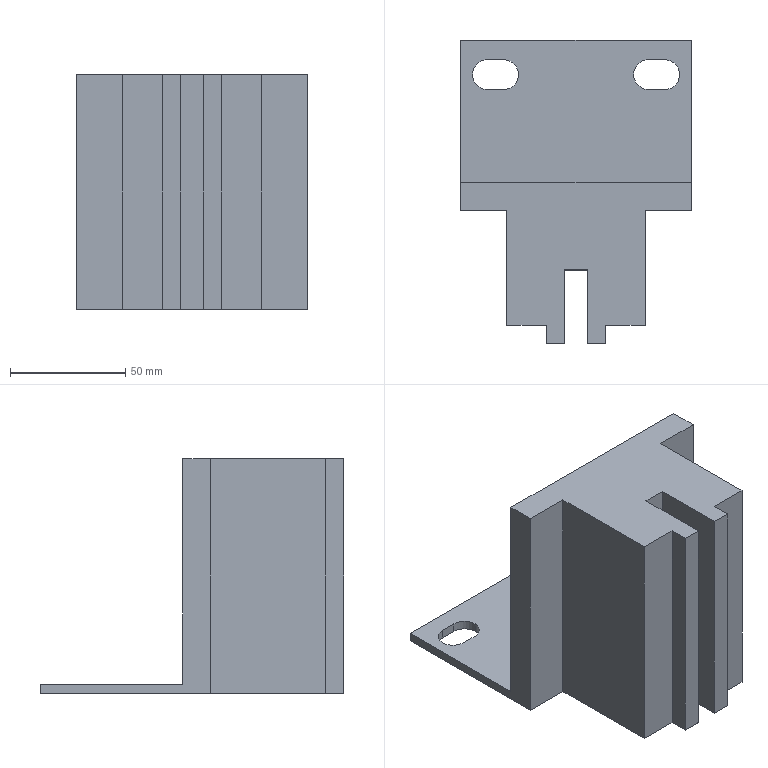Part | 1 solid | 30 faces | box 100 x 132 x 102 mm | volume 439986 mm3 | plane 24 | cylinder 6 | commonest cylinder face diameters 13 x6
STEP:
#1=CARTESIAN_POINT('',(45.,51.,0.));
#2=VERTEX_POINT('',#1);
#3=CARTESIAN_POINT('',(38.5,57.5,0.));
#4=VERTEX_POINT('',#3);
#5=CARTESIAN_POINT('',(38.5,51.,0.));
#6=DIRECTION('',(0.,0.,1.));
#7=DIRECTION('',(1.,0.,0.));
#8=AXIS2_PLACEMENT_3D('',#5,#6,#7);
#9=CIRCLE('',#8,6.5);
#10=EDGE_CURVE('',#2,#4,#9,.T.);
#11=ORIENTED_EDGE('',*,*,#10,.F.);
#12=CARTESIAN_POINT('',(45.,51.,4.));
#13=VERTEX_POINT('',#12);
#14=CARTESIAN_POINT('',(45.,51.,0.));
#15=DIRECTION('',(0.,0.,1.));
#16=VECTOR('',#15,1000.);
#17=LINE('',#14,#16);
#18=EDGE_CURVE('',#2,#13,#17,.T.);
#19=ORIENTED_EDGE('',*,*,#18,.T.);
#20=CARTESIAN_POINT('',(38.5,57.5,4.));
#21=VERTEX_POINT('',#20);
#22=CARTESIAN_POINT('',(38.5,51.,4.));
#23=DIRECTION('',(0.,0.,1.));
#24=DIRECTION('',(0.,1.,0.));
#25=AXIS2_PLACEMENT_3D('',#22,#23,#24);
#26=CIRCLE('',#25,6.5);
#27=EDGE_CURVE('',#13,#21,#26,.T.);
#28=ORIENTED_EDGE('',*,*,#27,.T.);
#29=CARTESIAN_POINT('',(38.5,57.5,0.));
#30=DIRECTION('',(0.,0.,1.));
#31=VECTOR('',#30,1000.);
#32=LINE('',#29,#31);
#33=EDGE_CURVE('',#4,#21,#32,.T.);
#34=ORIENTED_EDGE('',*,*,#33,.F.);
#35=EDGE_LOOP('',(#11,#19,#28,#34));
#36=FACE_OUTER_BOUND('',#35,.T.);
#37=CARTESIAN_POINT('',(38.5,51.,0.));
#38=DIRECTION('',(0.,0.,1.));
#39=DIRECTION('',(1.,0.,0.));
#40=AXIS2_PLACEMENT_3D('',#37,#38,#39);
#41=CYLINDRICAL_SURFACE('',#40,6.5);
#42=ADVANCED_FACE('',(#36),#41,.F.);
#43=CARTESIAN_POINT('',(-25.,51.,0.));
#44=VERTEX_POINT('',#43);
#45=CARTESIAN_POINT('',(-31.5,57.5,0.));
#46=VERTEX_POINT('',#45);
#47=CARTESIAN_POINT('',(-31.5,51.,0.));
#48=DIRECTION('',(0.,0.,1.));
#49=DIRECTION('',(-1.,0.,0.));
#50=AXIS2_PLACEMENT_3D('',#47,#48,#49);
#51=CIRCLE('',#50,6.5);
#52=EDGE_CURVE('',#44,#46,#51,.T.);
#53=ORIENTED_EDGE('',*,*,#52,.F.);
#54=CARTESIAN_POINT('',(-25.,51.,4.));
#55=VERTEX_POINT('',#54);
#56=CARTESIAN_POINT('',(-25.,51.,0.));
#57=DIRECTION('',(0.,0.,1.));
#58=VECTOR('',#57,1000.);
#59=LINE('',#56,#58);
#60=EDGE_CURVE('',#44,#55,#59,.T.);
#61=ORIENTED_EDGE('',*,*,#60,.T.);
#62=CARTESIAN_POINT('',(-31.5,57.5,4.));
#63=VERTEX_POINT('',#62);
#64=CARTESIAN_POINT('',(-31.5,51.,4.));
#65=DIRECTION('',(0.,0.,1.));
#66=DIRECTION('',(0.,1.,0.));
#67=AXIS2_PLACEMENT_3D('',#64,#65,#66);
#68=CIRCLE('',#67,6.5);
#69=EDGE_CURVE('',#55,#63,#68,.T.);
#70=ORIENTED_EDGE('',*,*,#69,.T.);
#71=CARTESIAN_POINT('',(-31.5,57.5,0.));
#72=DIRECTION('',(0.,0.,1.));
#73=VECTOR('',#72,1000.);
#74=LINE('',#71,#73);
#75=EDGE_CURVE('',#46,#63,#74,.T.);
#76=ORIENTED_EDGE('',*,*,#75,.F.);
#77=EDGE_LOOP('',(#53,#61,#70,#76));
#78=FACE_OUTER_BOUND('',#77,.T.);
#79=CARTESIAN_POINT('',(-31.5,51.,0.));
#80=DIRECTION('',(0.,0.,1.));
#81=DIRECTION('',(1.,0.,0.));
#82=AXIS2_PLACEMENT_3D('',#79,#80,#81);
#83=CYLINDRICAL_SURFACE('',#82,6.5);
#84=ADVANCED_FACE('',(#78),#83,.F.);
#85=CARTESIAN_POINT('',(5.,-66.,0.));
#86=VERTEX_POINT('',#85);
#87=CARTESIAN_POINT('',(13.,-66.,0.));
#88=VERTEX_POINT('',#87);
#89=CARTESIAN_POINT('',(-50.,-66.,0.));
#90=DIRECTION('',(1.,0.,0.));
#91=VECTOR('',#90,1000.);
#92=LINE('',#89,#91);
#93=EDGE_CURVE('',#86,#88,#92,.T.);
#94=ORIENTED_EDGE('',*,*,#93,.T.);
#95=CARTESIAN_POINT('',(13.,-66.,102.));
#96=VERTEX_POINT('',#95);
#97=CARTESIAN_POINT('',(13.,-66.,0.));
#98=DIRECTION('',(0.,0.,1.));
#99=VECTOR('',#98,1000.);
#100=LINE('',#97,#99);
#101=EDGE_CURVE('',#88,#96,#100,.T.);
#102=ORIENTED_EDGE('',*,*,#101,.T.);
#103=CARTESIAN_POINT('',(5.,-66.,102.));
#104=VERTEX_POINT('',#103);
#105=CARTESIAN_POINT('',(-50.,-66.,102.));
#106=DIRECTION('',(1.,0.,0.));
#107=VECTOR('',#106,1000.);
#108=LINE('',#105,#107);
#109=EDGE_CURVE('',#104,#96,#108,.T.);
#110=ORIENTED_EDGE('',*,*,#109,.F.);
#111=CARTESIAN_POINT('',(5.,-66.,102.));
#112=DIRECTION('',(0.,0.,-1.));
#113=VECTOR('',#112,1000.);
#114=LINE('',#111,#113);
#115=EDGE_CURVE('',#104,#86,#114,.T.);
#116=ORIENTED_EDGE('',*,*,#115,.T.);
#117=EDGE_LOOP('',(#94,#102,#110,#116));
#118=FACE_OUTER_BOUND('',#117,.T.);
#119=CARTESIAN_POINT('',(-50.,-66.,102.));
#120=DIRECTION('',(0.,1.,0.));
#121=DIRECTION('',(0.,0.,1.));
#122=AXIS2_PLACEMENT_3D('',#119,#120,#121);
#123=PLANE('',#122);
#124=ADVANCED_FACE('',(#118),#123,.F.);
#125=CARTESIAN_POINT('',(50.,-8.,102.));
#126=VERTEX_POINT('',#125);
#127=CARTESIAN_POINT('',(50.,4.,102.));
#128=VERTEX_POINT('',#127);
#129=CARTESIAN_POINT('',(50.,66.,102.));
#130=DIRECTION('',(0.,1.,0.));
#131=VECTOR('',#130,1000.);
#132=LINE('',#129,#131);
#133=EDGE_CURVE('',#126,#128,#132,.T.);
#134=ORIENTED_EDGE('',*,*,#133,.F.);
#135=CARTESIAN_POINT('',(50.,-8.,0.));
#136=VERTEX_POINT('',#135);
#137=CARTESIAN_POINT('',(50.,-8.,0.));
#138=DIRECTION('',(0.,0.,1.));
#139=VECTOR('',#138,1000.);
#140=LINE('',#137,#139);
#141=EDGE_CURVE('',#136,#126,#140,.T.);
#142=ORIENTED_EDGE('',*,*,#141,.F.);
#143=CARTESIAN_POINT('',(50.,66.,0.));
#144=VERTEX_POINT('',#143);
#145=CARTESIAN_POINT('',(50.,66.,0.));
#146=DIRECTION('',(0.,1.,0.));
#147=VECTOR('',#146,1000.);
#148=LINE('',#145,#147);
#149=EDGE_CURVE('',#136,#144,#148,.T.);
#150=ORIENTED_EDGE('',*,*,#149,.T.);
#151=CARTESIAN_POINT('',(50.,66.,4.));
#152=VERTEX_POINT('',#151);
#153=CARTESIAN_POINT('',(50.,66.,102.));
#154=DIRECTION('',(0.,0.,-1.));
#155=VECTOR('',#154,1000.);
#156=LINE('',#153,#155);
#157=EDGE_CURVE('',#152,#144,#156,.T.);
#158=ORIENTED_EDGE('',*,*,#157,.F.);
#159=CARTESIAN_POINT('',(50.,4.,4.));
#160=VERTEX_POINT('',#159);
#161=CARTESIAN_POINT('',(50.,66.,4.));
#162=DIRECTION('',(0.,-1.,0.));
#163=VECTOR('',#162,1000.);
#164=LINE('',#161,#163);
#165=EDGE_CURVE('',#152,#160,#164,.T.);
#166=ORIENTED_EDGE('',*,*,#165,.T.);
#167=CARTESIAN_POINT('',(50.,4.,102.));
#168=DIRECTION('',(0.,0.,1.));
#169=VECTOR('',#168,1000.);
#170=LINE('',#167,#169);
#171=EDGE_CURVE('',#160,#128,#170,.T.);
#172=ORIENTED_EDGE('',*,*,#171,.T.);
#173=EDGE_LOOP('',(#134,#142,#150,#158,#166,#172));
#174=FACE_OUTER_BOUND('',#173,.T.);
#175=CARTESIAN_POINT('',(50.,66.,102.));
#176=DIRECTION('',(-1.,0.,0.));
#177=DIRECTION('',(0.,-1.,0.));
#178=AXIS2_PLACEMENT_3D('',#175,#176,#177);
#179=PLANE('',#178);
#180=ADVANCED_FACE('',(#174),#179,.F.);
#181=CARTESIAN_POINT('',(-50.,66.,4.));
#182=VERTEX_POINT('',#181);
#183=CARTESIAN_POINT('',(-50.,66.,0.));
#184=VERTEX_POINT('',#183);
#185=CARTESIAN_POINT('',(-50.,66.,102.));
#186=DIRECTION('',(0.,0.,-1.));
#187=VECTOR('',#186,1000.);
#188=LINE('',#185,#187);
#189=EDGE_CURVE('',#182,#184,#188,.T.);
#190=ORIENTED_EDGE('',*,*,#189,.F.);
#191=CARTESIAN_POINT('',(50.,66.,4.));
#192=DIRECTION('',(-1.,0.,0.));
#193=VECTOR('',#192,1000.);
#194=LINE('',#191,#193);
#195=EDGE_CURVE('',#152,#182,#194,.T.);
#196=ORIENTED_EDGE('',*,*,#195,.F.);
#197=ORIENTED_EDGE('',*,*,#157,.T.);
#198=CARTESIAN_POINT('',(-50.,66.,0.));
#199=DIRECTION('',(-1.,0.,0.));
#200=VECTOR('',#199,1000.);
#201=LINE('',#198,#200);
#202=EDGE_CURVE('',#144,#184,#201,.T.);
#203=ORIENTED_EDGE('',*,*,#202,.T.);
#204=EDGE_LOOP('',(#190,#196,#197,#203));
#205=FACE_OUTER_BOUND('',#204,.T.);
#206=CARTESIAN_POINT('',(-50.,66.,102.));
#207=DIRECTION('',(0.,-1.,0.));
#208=DIRECTION('',(0.,0.,-1.));
#209=AXIS2_PLACEMENT_3D('',#206,#207,#208);
#210=PLANE('',#209);
#211=ADVANCED_FACE('',(#205),#210,.F.);
#212=CARTESIAN_POINT('',(-50.,-8.,0.));
#213=VERTEX_POINT('',#212);
#214=CARTESIAN_POINT('',(-50.,66.,0.));
#215=DIRECTION('',(0.,-1.,0.));
#216=VECTOR('',#215,1000.);
#217=LINE('',#214,#216);
#218=EDGE_CURVE('',#184,#213,#217,.T.);
#219=ORIENTED_EDGE('',*,*,#218,.T.);
#220=CARTESIAN_POINT('',(-50.,-8.,102.));
#221=VERTEX_POINT('',#220);
#222=CARTESIAN_POINT('',(-50.,-8.,0.));
#223=DIRECTION('',(0.,0.,1.));
#224=VECTOR('',#223,1000.);
#225=LINE('',#222,#224);
#226=EDGE_CURVE('',#213,#221,#225,.T.);
#227=ORIENTED_EDGE('',*,*,#226,.T.);
#228=CARTESIAN_POINT('',(-50.,4.,102.));
#229=VERTEX_POINT('',#228);
#230=CARTESIAN_POINT('',(-50.,66.,102.));
#231=DIRECTION('',(0.,-1.,0.));
#232=VECTOR('',#231,1000.);
#233=LINE('',#230,#232);
#234=EDGE_CURVE('',#229,#221,#233,.T.);
#235=ORIENTED_EDGE('',*,*,#234,.F.);
#236=CARTESIAN_POINT('',(-50.,4.,4.));
#237=VERTEX_POINT('',#236);
#238=CARTESIAN_POINT('',(-50.,4.,102.));
#239=DIRECTION('',(0.,0.,-1.));
#240=VECTOR('',#239,1000.);
#241=LINE('',#238,#240);
#242=EDGE_CURVE('',#229,#237,#241,.T.);
#243=ORIENTED_EDGE('',*,*,#242,.T.);
#244=CARTESIAN_POINT('',(-50.,66.,4.));
#245=DIRECTION('',(0.,1.,0.));
#246=VECTOR('',#245,1000.);
#247=LINE('',#244,#246);
#248=EDGE_CURVE('',#237,#182,#247,.T.);
#249=ORIENTED_EDGE('',*,*,#248,.T.);
#250=ORIENTED_EDGE('',*,*,#189,.T.);
#251=EDGE_LOOP('',(#219,#227,#235,#243,#249,#250));
#252=FACE_OUTER_BOUND('',#251,.T.);
#253=CARTESIAN_POINT('',(-50.,66.,102.));
#254=DIRECTION('',(1.,0.,0.));
#255=DIRECTION('',(0.,1.,0.));
#256=AXIS2_PLACEMENT_3D('',#253,#254,#255);
#257=PLANE('',#256);
#258=ADVANCED_FACE('',(#252),#257,.F.);
#259=CARTESIAN_POINT('',(-13.,-66.,102.));
#260=VERTEX_POINT('',#259);
#261=CARTESIAN_POINT('',(-5.,-66.,102.));
#262=VERTEX_POINT('',#261);
#263=CARTESIAN_POINT('',(-50.,-66.,102.));
#264=DIRECTION('',(1.,0.,0.));
#265=VECTOR('',#264,1000.);
#266=LINE('',#263,#265);
#267=EDGE_CURVE('',#260,#262,#266,.T.);
#268=ORIENTED_EDGE('',*,*,#267,.F.);
#269=CARTESIAN_POINT('',(-13.,-66.,0.));
#270=VERTEX_POINT('',#269);
#271=CARTESIAN_POINT('',(-13.,-66.,0.));
#272=DIRECTION('',(0.,0.,1.));
#273=VECTOR('',#272,1000.);
#274=LINE('',#271,#273);
#275=EDGE_CURVE('',#270,#260,#274,.T.);
#276=ORIENTED_EDGE('',*,*,#275,.F.);
#277=CARTESIAN_POINT('',(-5.,-66.,0.));
#278=VERTEX_POINT('',#277);
#279=CARTESIAN_POINT('',(-50.,-66.,0.));
#280=DIRECTION('',(1.,0.,0.));
#281=VECTOR('',#280,1000.);
#282=LINE('',#279,#281);
#283=EDGE_CURVE('',#270,#278,#282,.T.);
#284=ORIENTED_EDGE('',*,*,#283,.T.);
#285=CARTESIAN_POINT('',(-5.,-66.,102.));
#286=DIRECTION('',(0.,0.,1.));
#287=VECTOR('',#286,1000.);
#288=LINE('',#285,#287);
#289=EDGE_CURVE('',#278,#262,#288,.T.);
#290=ORIENTED_EDGE('',*,*,#289,.T.);
#291=EDGE_LOOP('',(#268,#276,#284,#290));
#292=FACE_OUTER_BOUND('',#291,.T.);
#293=CARTESIAN_POINT('',(-50.,-66.,102.));
#294=DIRECTION('',(0.,1.,0.));
#295=DIRECTION('',(0.,0.,1.));
#296=AXIS2_PLACEMENT_3D('',#293,#294,#295);
#297=PLANE('',#296);
#298=ADVANCED_FACE('',(#292),#297,.F.);
#299=CARTESIAN_POINT('',(-30.,-8.,102.));
#300=VERTEX_POINT('',#299);
#301=CARTESIAN_POINT('',(0.,-8.,102.));
#302=DIRECTION('',(-1.,0.,0.));
#303=VECTOR('',#302,1000.);
#304=LINE('',#301,#303);
#305=EDGE_CURVE('',#300,#221,#304,.T.);
#306=ORIENTED_EDGE('',*,*,#305,.F.);
#307=CARTESIAN_POINT('',(-30.,-58.,102.));
#308=VERTEX_POINT('',#307);
#309=CARTESIAN_POINT('',(-30.,0.,102.));
#310=DIRECTION('',(0.,1.,0.));
#311=VECTOR('',#310,1000.);
#312=LINE('',#309,#311);
#313=EDGE_CURVE('',#308,#300,#312,.T.);
#314=ORIENTED_EDGE('',*,*,#313,.F.);
#315=CARTESIAN_POINT('',(-13.,-58.,102.));
#316=VERTEX_POINT('',#315);
#317=CARTESIAN_POINT('',(0.,-58.,102.));
#318=DIRECTION('',(-1.,0.,0.));
#319=VECTOR('',#318,1000.);
#320=LINE('',#317,#319);
#321=EDGE_CURVE('',#316,#308,#320,.T.);
#322=ORIENTED_EDGE('',*,*,#321,.F.);
#323=CARTESIAN_POINT('',(-13.,0.,102.));
#324=DIRECTION('',(0.,1.,0.));
#325=VECTOR('',#324,1000.);
#326=LINE('',#323,#325);
#327=EDGE_CURVE('',#260,#316,#326,.T.);
#328=ORIENTED_EDGE('',*,*,#327,.F.);
#329=ORIENTED_EDGE('',*,*,#267,.T.);
#330=CARTESIAN_POINT('',(-5.,-34.,102.));
#331=VERTEX_POINT('',#330);
#332=CARTESIAN_POINT('',(-5.,0.,102.));
#333=DIRECTION('',(0.,-1.,0.));
#334=VECTOR('',#333,1000.);
#335=LINE('',#332,#334);
#336=EDGE_CURVE('',#331,#262,#335,.T.);
#337=ORIENTED_EDGE('',*,*,#336,.F.);
#338=CARTESIAN_POINT('',(5.,-34.,102.));
#339=VERTEX_POINT('',#338);
#340=CARTESIAN_POINT('',(0.,-34.,102.));
#341=DIRECTION('',(-1.,0.,0.));
#342=VECTOR('',#341,1000.);
#343=LINE('',#340,#342);
#344=EDGE_CURVE('',#339,#331,#343,.T.);
#345=ORIENTED_EDGE('',*,*,#344,.F.);
#346=CARTESIAN_POINT('',(5.,0.,102.));
#347=DIRECTION('',(0.,1.,0.));
#348=VECTOR('',#347,1000.);
#349=LINE('',#346,#348);
#350=EDGE_CURVE('',#104,#339,#349,.T.);
#351=ORIENTED_EDGE('',*,*,#350,.F.);
#352=ORIENTED_EDGE('',*,*,#109,.T.);
#353=CARTESIAN_POINT('',(13.,-58.,102.));
#354=VERTEX_POINT('',#353);
#355=CARTESIAN_POINT('',(13.,0.,102.));
#356=DIRECTION('',(0.,-1.,0.));
#357=VECTOR('',#356,1000.);
#358=LINE('',#355,#357);
#359=EDGE_CURVE('',#354,#96,#358,.T.);
#360=ORIENTED_EDGE('',*,*,#359,.F.);
#361=CARTESIAN_POINT('',(30.,-58.,102.));
#362=VERTEX_POINT('',#361);
#363=CARTESIAN_POINT('',(0.,-58.,102.));
#364=DIRECTION('',(-1.,0.,0.));
#365=VECTOR('',#364,1000.);
#366=LINE('',#363,#365);
#367=EDGE_CURVE('',#362,#354,#366,.T.);
#368=ORIENTED_EDGE('',*,*,#367,.F.);
#369=CARTESIAN_POINT('',(30.,-8.,102.));
#370=VERTEX_POINT('',#369);
#371=CARTESIAN_POINT('',(30.,0.,102.));
#372=DIRECTION('',(0.,-1.,0.));
#373=VECTOR('',#372,1000.);
#374=LINE('',#371,#373);
#375=EDGE_CURVE('',#370,#362,#374,.T.);
#376=ORIENTED_EDGE('',*,*,#375,.F.);
#377=CARTESIAN_POINT('',(0.,-8.,102.));
#378=DIRECTION('',(-1.,0.,0.));
#379=VECTOR('',#378,1000.);
#380=LINE('',#377,#379);
#381=EDGE_CURVE('',#126,#370,#380,.T.);
#382=ORIENTED_EDGE('',*,*,#381,.F.);
#383=ORIENTED_EDGE('',*,*,#133,.T.);
#384=CARTESIAN_POINT('',(50.,4.,102.));
#385=DIRECTION('',(-1.,0.,0.));
#386=VECTOR('',#385,1000.);
#387=LINE('',#384,#386);
#388=EDGE_CURVE('',#128,#229,#387,.T.);
#389=ORIENTED_EDGE('',*,*,#388,.T.);
#390=ORIENTED_EDGE('',*,*,#234,.T.);
#391=EDGE_LOOP('',(#306,#314,#322,#328,#329,#337,#345,#351,#352,#360,#368,#376,#382,#383,#389,#390));
#392=FACE_OUTER_BOUND('',#391,.T.);
#393=CARTESIAN_POINT('',(0.,0.,102.));
#394=DIRECTION('',(0.,0.,1.));
#395=DIRECTION('',(1.,0.,0.));
#396=AXIS2_PLACEMENT_3D('',#393,#394,#395);
#397=PLANE('',#396);
#398=ADVANCED_FACE('',(#392),#397,.T.);
#399=CARTESIAN_POINT('',(31.5,57.5,0.));
#400=VERTEX_POINT('',#399);
#401=CARTESIAN_POINT('',(31.5,57.5,0.));
#402=DIRECTION('',(-1.,0.,0.));
#403=VECTOR('',#402,1000.);
#404=LINE('',#401,#403);
#405=EDGE_CURVE('',#4,#400,#404,.T.);
#406=ORIENTED_EDGE('',*,*,#405,.T.);
#407=CARTESIAN_POINT('',(31.5,44.5,0.));
#408=VERTEX_POINT('',#407);
#409=CARTESIAN_POINT('',(31.5,51.,0.));
#410=DIRECTION('',(0.,0.,1.));
#411=DIRECTION('',(1.,0.,0.));
#412=AXIS2_PLACEMENT_3D('',#409,#410,#411);
#413=CIRCLE('',#412,6.5);
#414=EDGE_CURVE('',#400,#408,#413,.T.);
#415=ORIENTED_EDGE('',*,*,#414,.T.);
#416=CARTESIAN_POINT('',(38.5,44.5,0.));
#417=VERTEX_POINT('',#416);
#418=CARTESIAN_POINT('',(31.5,44.5,0.));
#419=DIRECTION('',(1.,0.,0.));
#420=VECTOR('',#419,1000.);
#421=LINE('',#418,#420);
#422=EDGE_CURVE('',#408,#417,#421,.T.);
#423=ORIENTED_EDGE('',*,*,#422,.T.);
#424=CARTESIAN_POINT('',(38.5,51.,0.));
#425=DIRECTION('',(0.,0.,1.));
#426=DIRECTION('',(1.,0.,0.));
#427=AXIS2_PLACEMENT_3D('',#424,#425,#426);
#428=CIRCLE('',#427,6.5);
#429=EDGE_CURVE('',#417,#2,#428,.T.);
#430=ORIENTED_EDGE('',*,*,#429,.T.);
#431=ORIENTED_EDGE('',*,*,#10,.T.);
#432=EDGE_LOOP('',(#406,#415,#423,#430,#431));
#433=FACE_BOUND('',#432,.T.);
#434=CARTESIAN_POINT('',(-38.5,44.5,0.));
#435=VERTEX_POINT('',#434);
#436=CARTESIAN_POINT('',(-31.5,44.5,0.));
#437=VERTEX_POINT('',#436);
#438=CARTESIAN_POINT('',(-31.5,44.5,0.));
#439=DIRECTION('',(1.,0.,0.));
#440=VECTOR('',#439,1000.);
#441=LINE('',#438,#440);
#442=EDGE_CURVE('',#435,#437,#441,.T.);
#443=ORIENTED_EDGE('',*,*,#442,.T.);
#444=CARTESIAN_POINT('',(-31.5,51.,0.));
#445=DIRECTION('',(0.,0.,1.));
#446=DIRECTION('',(-1.,0.,0.));
#447=AXIS2_PLACEMENT_3D('',#444,#445,#446);
#448=CIRCLE('',#447,6.5);
#449=EDGE_CURVE('',#437,#44,#448,.T.);
#450=ORIENTED_EDGE('',*,*,#449,.T.);
#451=ORIENTED_EDGE('',*,*,#52,.T.);
#452=CARTESIAN_POINT('',(-38.5,57.5,0.));
#453=VERTEX_POINT('',#452);
#454=CARTESIAN_POINT('',(-31.5,57.5,0.));
#455=DIRECTION('',(-1.,0.,0.));
#456=VECTOR('',#455,1000.);
#457=LINE('',#454,#456);
#458=EDGE_CURVE('',#46,#453,#457,.T.);
#459=ORIENTED_EDGE('',*,*,#458,.T.);
#460=CARTESIAN_POINT('',(-38.5,51.,0.));
#461=DIRECTION('',(0.,0.,1.));
#462=DIRECTION('',(-1.,0.,0.));
#463=AXIS2_PLACEMENT_3D('',#460,#461,#462);
#464=CIRCLE('',#463,6.5);
#465=EDGE_CURVE('',#453,#435,#464,.T.);
#466=ORIENTED_EDGE('',*,*,#465,.T.);
#467=EDGE_LOOP('',(#443,#450,#451,#459,#466));
#468=FACE_BOUND('',#467,.T.);
#469=CARTESIAN_POINT('',(-30.,-58.,0.));
#470=VERTEX_POINT('',#469);
#471=CARTESIAN_POINT('',(-30.,-8.,0.));
#472=VERTEX_POINT('',#471);
#473=CARTESIAN_POINT('',(-30.,-58.,0.));
#474=DIRECTION('',(0.,1.,0.));
#475=VECTOR('',#474,1000.);
#476=LINE('',#473,#475);
#477=EDGE_CURVE('',#470,#472,#476,.T.);
#478=ORIENTED_EDGE('',*,*,#477,.T.);
#479=CARTESIAN_POINT('',(-50.,-8.,0.));
#480=DIRECTION('',(-1.,0.,0.));
#481=VECTOR('',#480,1000.);
#482=LINE('',#479,#481);
#483=EDGE_CURVE('',#472,#213,#482,.T.);
#484=ORIENTED_EDGE('',*,*,#483,.T.);
#485=ORIENTED_EDGE('',*,*,#218,.F.);
#486=ORIENTED_EDGE('',*,*,#202,.F.);
#487=ORIENTED_EDGE('',*,*,#149,.F.);
#488=CARTESIAN_POINT('',(30.,-8.,0.));
#489=VERTEX_POINT('',#488);
#490=CARTESIAN_POINT('',(50.,-8.,0.));
#491=DIRECTION('',(-1.,0.,0.));
#492=VECTOR('',#491,1000.);
#493=LINE('',#490,#492);
#494=EDGE_CURVE('',#136,#489,#493,.T.);
#495=ORIENTED_EDGE('',*,*,#494,.T.);
#496=CARTESIAN_POINT('',(30.,-58.,0.));
#497=VERTEX_POINT('',#496);
#498=CARTESIAN_POINT('',(30.,-58.,0.));
#499=DIRECTION('',(0.,-1.,0.));
#500=VECTOR('',#499,1000.);
#501=LINE('',#498,#500);
#502=EDGE_CURVE('',#489,#497,#501,.T.);
#503=ORIENTED_EDGE('',*,*,#502,.T.);
#504=CARTESIAN_POINT('',(13.,-58.,0.));
#505=VERTEX_POINT('',#504);
#506=CARTESIAN_POINT('',(50.,-58.,0.));
#507=DIRECTION('',(-1.,0.,0.));
#508=VECTOR('',#507,1000.);
#509=LINE('',#506,#508);
#510=EDGE_CURVE('',#497,#505,#509,.T.);
#511=ORIENTED_EDGE('',*,*,#510,.T.);
#512=CARTESIAN_POINT('',(13.,-66.,0.));
#513=DIRECTION('',(0.,-1.,0.));
#514=VECTOR('',#513,1000.);
#515=LINE('',#512,#514);
#516=EDGE_CURVE('',#505,#88,#515,.T.);
#517=ORIENTED_EDGE('',*,*,#516,.T.);
#518=ORIENTED_EDGE('',*,*,#93,.F.);
#519=CARTESIAN_POINT('',(5.,-34.,0.));
#520=VERTEX_POINT('',#519);
#521=CARTESIAN_POINT('',(5.,0.,0.));
#522=DIRECTION('',(0.,1.,0.));
#523=VECTOR('',#522,1000.);
#524=LINE('',#521,#523);
#525=EDGE_CURVE('',#86,#520,#524,.T.);
#526=ORIENTED_EDGE('',*,*,#525,.T.);
#527=CARTESIAN_POINT('',(-5.,-34.,0.));
#528=VERTEX_POINT('',#527);
#529=CARTESIAN_POINT('',(-5.,-34.,0.));
#530=DIRECTION('',(-1.,0.,0.));
#531=VECTOR('',#530,1000.);
#532=LINE('',#529,#531);
#533=EDGE_CURVE('',#520,#528,#532,.T.);
#534=ORIENTED_EDGE('',*,*,#533,.T.);
#535=CARTESIAN_POINT('',(-5.,-98.,0.));
#536=DIRECTION('',(0.,-1.,0.));
#537=VECTOR('',#536,1000.);
#538=LINE('',#535,#537);
#539=EDGE_CURVE('',#528,#278,#538,.T.);
#540=ORIENTED_EDGE('',*,*,#539,.T.);
#541=ORIENTED_EDGE('',*,*,#283,.F.);
#542=CARTESIAN_POINT('',(-13.,-58.,0.));
#543=VERTEX_POINT('',#542);
#544=CARTESIAN_POINT('',(-13.,-66.,0.));
#545=DIRECTION('',(0.,1.,0.));
#546=VECTOR('',#545,1000.);
#547=LINE('',#544,#546);
#548=EDGE_CURVE('',#270,#543,#547,.T.);
#549=ORIENTED_EDGE('',*,*,#548,.T.);
#550=CARTESIAN_POINT('',(-50.,-58.,0.));
#551=DIRECTION('',(-1.,0.,0.));
#552=VECTOR('',#551,1000.);
#553=LINE('',#550,#552);
#554=EDGE_CURVE('',#543,#470,#553,.T.);
#555=ORIENTED_EDGE('',*,*,#554,.T.);
#556=EDGE_LOOP('',(#478,#484,#485,#486,#487,#495,#503,#511,#517,#518,#526,#534,#540,#541,#549,#555));
#557=FACE_OUTER_BOUND('',#556,.T.);
#558=CARTESIAN_POINT('',(0.,0.,0.));
#559=DIRECTION('',(0.,0.,1.));
#560=DIRECTION('',(1.,0.,0.));
#561=AXIS2_PLACEMENT_3D('',#558,#559,#560);
#562=PLANE('',#561);
#563=ADVANCED_FACE('',(#433,#468,#557),#562,.F.);
#564=ORIENTED_EDGE('',*,*,#350,.T.);
#565=CARTESIAN_POINT('',(5.,-34.,0.));
#566=DIRECTION('',(0.,0.,1.));
#567=VECTOR('',#566,1000.);
#568=LINE('',#565,#567);
#569=EDGE_CURVE('',#520,#339,#568,.T.);
#570=ORIENTED_EDGE('',*,*,#569,.F.);
#571=ORIENTED_EDGE('',*,*,#525,.F.);
#572=ORIENTED_EDGE('',*,*,#115,.F.);
#573=EDGE_LOOP('',(#564,#570,#571,#572));
#574=FACE_OUTER_BOUND('',#573,.T.);
#575=CARTESIAN_POINT('',(5.,-98.,0.));
#576=DIRECTION('',(1.,0.,0.));
#577=DIRECTION('',(0.,1.,0.));
#578=AXIS2_PLACEMENT_3D('',#575,#576,#577);
#579=PLANE('',#578);
#580=ADVANCED_FACE('',(#574),#579,.F.);
#581=ORIENTED_EDGE('',*,*,#539,.F.);
#582=CARTESIAN_POINT('',(-5.,-34.,0.));
#583=DIRECTION('',(0.,0.,1.));
#584=VECTOR('',#583,1000.);
#585=LINE('',#582,#584);
#586=EDGE_CURVE('',#528,#331,#585,.T.);
#587=ORIENTED_EDGE('',*,*,#586,.T.);
#588=ORIENTED_EDGE('',*,*,#336,.T.);
#589=ORIENTED_EDGE('',*,*,#289,.F.);
#590=EDGE_LOOP('',(#581,#587,#588,#589));
#591=FACE_OUTER_BOUND('',#590,.T.);
#592=CARTESIAN_POINT('',(-5.,-98.,0.));
#593=DIRECTION('',(-1.,0.,0.));
#594=DIRECTION('',(0.,0.,1.));
#595=AXIS2_PLACEMENT_3D('',#592,#593,#594);
#596=PLANE('',#595);
#597=ADVANCED_FACE('',(#591),#596,.F.);
#598=ORIENTED_EDGE('',*,*,#344,.T.);
#599=ORIENTED_EDGE('',*,*,#586,.F.);
#600=ORIENTED_EDGE('',*,*,#533,.F.);
#601=ORIENTED_EDGE('',*,*,#569,.T.);
#602=EDGE_LOOP('',(#598,#599,#600,#601));
#603=FACE_OUTER_BOUND('',#602,.T.);
#604=CARTESIAN_POINT('',(-5.,-34.,0.));
#605=DIRECTION('',(0.,1.,0.));
#606=DIRECTION('',(-1.,0.,0.));
#607=AXIS2_PLACEMENT_3D('',#604,#605,#606);
#608=PLANE('',#607);
#609=ADVANCED_FACE('',(#603),#608,.F.);
#610=ORIENTED_EDGE('',*,*,#60,.F.);
#611=ORIENTED_EDGE('',*,*,#449,.F.);
#612=CARTESIAN_POINT('',(-31.5,44.5,4.));
#613=VERTEX_POINT('',#612);
#614=CARTESIAN_POINT('',(-31.5,44.5,0.));
#615=DIRECTION('',(0.,0.,1.));
#616=VECTOR('',#615,1000.);
#617=LINE('',#614,#616);
#618=EDGE_CURVE('',#437,#613,#617,.T.);
#619=ORIENTED_EDGE('',*,*,#618,.T.);
#620=CARTESIAN_POINT('',(-31.5,51.,4.));
#621=DIRECTION('',(0.,0.,1.));
#622=DIRECTION('',(0.,1.,0.));
#623=AXIS2_PLACEMENT_3D('',#620,#621,#622);
#624=CIRCLE('',#623,6.5);
#625=EDGE_CURVE('',#613,#55,#624,.T.);
#626=ORIENTED_EDGE('',*,*,#625,.T.);
#627=EDGE_LOOP('',(#610,#611,#619,#626));
#628=FACE_OUTER_BOUND('',#627,.T.);
#629=CARTESIAN_POINT('',(-31.5,51.,0.));
#630=DIRECTION('',(0.,0.,1.));
#631=DIRECTION('',(1.,0.,0.));
#632=AXIS2_PLACEMENT_3D('',#629,#630,#631);
#633=CYLINDRICAL_SURFACE('',#632,6.5);
#634=ADVANCED_FACE('',(#628),#633,.F.);
#635=CARTESIAN_POINT('',(-38.5,44.5,4.));
#636=VERTEX_POINT('',#635);
#637=CARTESIAN_POINT('',(-38.5,44.5,0.));
#638=DIRECTION('',(0.,0.,1.));
#639=VECTOR('',#638,1000.);
#640=LINE('',#637,#639);
#641=EDGE_CURVE('',#435,#636,#640,.T.);
#642=ORIENTED_EDGE('',*,*,#641,.T.);
#643=CARTESIAN_POINT('',(-31.5,44.5,4.));
#644=DIRECTION('',(1.,0.,0.));
#645=VECTOR('',#644,1000.);
#646=LINE('',#643,#645);
#647=EDGE_CURVE('',#636,#613,#646,.T.);
#648=ORIENTED_EDGE('',*,*,#647,.T.);
#649=ORIENTED_EDGE('',*,*,#618,.F.);
#650=ORIENTED_EDGE('',*,*,#442,.F.);
#651=EDGE_LOOP('',(#642,#648,#649,#650));
#652=FACE_OUTER_BOUND('',#651,.T.);
#653=CARTESIAN_POINT('',(-31.5,44.5,0.));
#654=DIRECTION('',(0.,-1.,0.));
#655=DIRECTION('',(0.,0.,-1.));
#656=AXIS2_PLACEMENT_3D('',#653,#654,#655);
#657=PLANE('',#656);
#658=ADVANCED_FACE('',(#652),#657,.F.);
#659=CARTESIAN_POINT('',(-38.5,57.5,4.));
#660=VERTEX_POINT('',#659);
#661=CARTESIAN_POINT('',(-38.5,57.5,0.));
#662=DIRECTION('',(0.,0.,1.));
#663=VECTOR('',#662,1000.);
#664=LINE('',#661,#663);
#665=EDGE_CURVE('',#453,#660,#664,.T.);
#666=ORIENTED_EDGE('',*,*,#665,.T.);
#667=CARTESIAN_POINT('',(-38.5,51.,4.));
#668=DIRECTION('',(0.,0.,1.));
#669=DIRECTION('',(0.,1.,0.));
#670=AXIS2_PLACEMENT_3D('',#667,#668,#669);
#671=CIRCLE('',#670,6.5);
#672=EDGE_CURVE('',#660,#636,#671,.T.);
#673=ORIENTED_EDGE('',*,*,#672,.T.);
#674=ORIENTED_EDGE('',*,*,#641,.F.);
#675=ORIENTED_EDGE('',*,*,#465,.F.);
#676=EDGE_LOOP('',(#666,#673,#674,#675));
#677=FACE_OUTER_BOUND('',#676,.T.);
#678=CARTESIAN_POINT('',(-38.5,51.,0.));
#679=DIRECTION('',(0.,0.,1.));
#680=DIRECTION('',(1.,0.,0.));
#681=AXIS2_PLACEMENT_3D('',#678,#679,#680);
#682=CYLINDRICAL_SURFACE('',#681,6.5);
#683=ADVANCED_FACE('',(#677),#682,.F.);
#684=ORIENTED_EDGE('',*,*,#75,.T.);
#685=CARTESIAN_POINT('',(-31.5,57.5,4.));
#686=DIRECTION('',(-1.,0.,0.));
#687=VECTOR('',#686,1000.);
#688=LINE('',#685,#687);
#689=EDGE_CURVE('',#63,#660,#688,.T.);
#690=ORIENTED_EDGE('',*,*,#689,.T.);
#691=ORIENTED_EDGE('',*,*,#665,.F.);
#692=ORIENTED_EDGE('',*,*,#458,.F.);
#693=EDGE_LOOP('',(#684,#690,#691,#692));
#694=FACE_OUTER_BOUND('',#693,.T.);
#695=CARTESIAN_POINT('',(-31.5,57.5,0.));
#696=DIRECTION('',(0.,1.,0.));
#697=DIRECTION('',(0.,0.,1.));
#698=AXIS2_PLACEMENT_3D('',#695,#696,#697);
#699=PLANE('',#698);
#700=ADVANCED_FACE('',(#694),#699,.F.);
#701=CARTESIAN_POINT('',(31.5,57.5,4.));
#702=VERTEX_POINT('',#701);
#703=CARTESIAN_POINT('',(31.5,57.5,0.));
#704=DIRECTION('',(0.,0.,1.));
#705=VECTOR('',#704,1000.);
#706=LINE('',#703,#705);
#707=EDGE_CURVE('',#400,#702,#706,.T.);
#708=ORIENTED_EDGE('',*,*,#707,.T.);
#709=CARTESIAN_POINT('',(31.5,44.5,4.));
#710=VERTEX_POINT('',#709);
#711=CARTESIAN_POINT('',(31.5,51.,4.));
#712=DIRECTION('',(0.,0.,1.));
#713=DIRECTION('',(0.,1.,0.));
#714=AXIS2_PLACEMENT_3D('',#711,#712,#713);
#715=CIRCLE('',#714,6.5);
#716=EDGE_CURVE('',#702,#710,#715,.T.);
#717=ORIENTED_EDGE('',*,*,#716,.T.);
#718=CARTESIAN_POINT('',(31.5,44.5,0.));
#719=DIRECTION('',(0.,0.,1.));
#720=VECTOR('',#719,1000.);
#721=LINE('',#718,#720);
#722=EDGE_CURVE('',#408,#710,#721,.T.);
#723=ORIENTED_EDGE('',*,*,#722,.F.);
#724=ORIENTED_EDGE('',*,*,#414,.F.);
#725=EDGE_LOOP('',(#708,#717,#723,#724));
#726=FACE_OUTER_BOUND('',#725,.T.);
#727=CARTESIAN_POINT('',(31.5,51.,0.));
#728=DIRECTION('',(0.,0.,1.));
#729=DIRECTION('',(1.,0.,0.));
#730=AXIS2_PLACEMENT_3D('',#727,#728,#729);
#731=CYLINDRICAL_SURFACE('',#730,6.5);
#732=ADVANCED_FACE('',(#726),#731,.F.);
#733=ORIENTED_EDGE('',*,*,#33,.T.);
#734=CARTESIAN_POINT('',(31.5,57.5,4.));
#735=DIRECTION('',(-1.,0.,0.));
#736=VECTOR('',#735,1000.);
#737=LINE('',#734,#736);
#738=EDGE_CURVE('',#21,#702,#737,.T.);
#739=ORIENTED_EDGE('',*,*,#738,.T.);
#740=ORIENTED_EDGE('',*,*,#707,.F.);
#741=ORIENTED_EDGE('',*,*,#405,.F.);
#742=EDGE_LOOP('',(#733,#739,#740,#741));
#743=FACE_OUTER_BOUND('',#742,.T.);
#744=CARTESIAN_POINT('',(31.5,57.5,0.));
#745=DIRECTION('',(0.,1.,0.));
#746=DIRECTION('',(0.,0.,1.));
#747=AXIS2_PLACEMENT_3D('',#744,#745,#746);
#748=PLANE('',#747);
#749=ADVANCED_FACE('',(#743),#748,.F.);
#750=ORIENTED_EDGE('',*,*,#18,.F.);
#751=ORIENTED_EDGE('',*,*,#429,.F.);
#752=CARTESIAN_POINT('',(38.5,44.5,4.));
#753=VERTEX_POINT('',#752);
#754=CARTESIAN_POINT('',(38.5,44.5,0.));
#755=DIRECTION('',(0.,0.,1.));
#756=VECTOR('',#755,1000.);
#757=LINE('',#754,#756);
#758=EDGE_CURVE('',#417,#753,#757,.T.);
#759=ORIENTED_EDGE('',*,*,#758,.T.);
#760=CARTESIAN_POINT('',(38.5,51.,4.));
#761=DIRECTION('',(0.,0.,1.));
#762=DIRECTION('',(0.,1.,0.));
#763=AXIS2_PLACEMENT_3D('',#760,#761,#762);
#764=CIRCLE('',#763,6.5);
#765=EDGE_CURVE('',#753,#13,#764,.T.);
#766=ORIENTED_EDGE('',*,*,#765,.T.);
#767=EDGE_LOOP('',(#750,#751,#759,#766));
#768=FACE_OUTER_BOUND('',#767,.T.);
#769=CARTESIAN_POINT('',(38.5,51.,0.));
#770=DIRECTION('',(0.,0.,1.));
#771=DIRECTION('',(1.,0.,0.));
#772=AXIS2_PLACEMENT_3D('',#769,#770,#771);
#773=CYLINDRICAL_SURFACE('',#772,6.5);
#774=ADVANCED_FACE('',(#768),#773,.F.);
#775=ORIENTED_EDGE('',*,*,#722,.T.);
#776=CARTESIAN_POINT('',(31.5,44.5,4.));
#777=DIRECTION('',(1.,0.,0.));
#778=VECTOR('',#777,1000.);
#779=LINE('',#776,#778);
#780=EDGE_CURVE('',#710,#753,#779,.T.);
#781=ORIENTED_EDGE('',*,*,#780,.T.);
#782=ORIENTED_EDGE('',*,*,#758,.F.);
#783=ORIENTED_EDGE('',*,*,#422,.F.);
#784=EDGE_LOOP('',(#775,#781,#782,#783));
#785=FACE_OUTER_BOUND('',#784,.T.);
#786=CARTESIAN_POINT('',(31.5,44.5,0.));
#787=DIRECTION('',(0.,-1.,0.));
#788=DIRECTION('',(0.,0.,-1.));
#789=AXIS2_PLACEMENT_3D('',#786,#787,#788);
#790=PLANE('',#789);
#791=ADVANCED_FACE('',(#785),#790,.F.);
#792=ORIENTED_EDGE('',*,*,#388,.F.);
#793=ORIENTED_EDGE('',*,*,#171,.F.);
#794=CARTESIAN_POINT('',(50.,4.,4.));
#795=DIRECTION('',(-1.,0.,0.));
#796=VECTOR('',#795,1000.);
#797=LINE('',#794,#796);
#798=EDGE_CURVE('',#160,#237,#797,.T.);
#799=ORIENTED_EDGE('',*,*,#798,.T.);
#800=ORIENTED_EDGE('',*,*,#242,.F.);
#801=EDGE_LOOP('',(#792,#793,#799,#800));
#802=FACE_OUTER_BOUND('',#801,.T.);
#803=CARTESIAN_POINT('',(50.,4.,102.));
#804=DIRECTION('',(0.,-1.,0.));
#805=DIRECTION('',(1.,0.,0.));
#806=AXIS2_PLACEMENT_3D('',#803,#804,#805);
#807=PLANE('',#806);
#808=ADVANCED_FACE('',(#802),#807,.F.);
#809=ORIENTED_EDGE('',*,*,#738,.F.);
#810=ORIENTED_EDGE('',*,*,#27,.F.);
#811=ORIENTED_EDGE('',*,*,#765,.F.);
#812=ORIENTED_EDGE('',*,*,#780,.F.);
#813=ORIENTED_EDGE('',*,*,#716,.F.);
#814=EDGE_LOOP('',(#809,#810,#811,#812,#813));
#815=FACE_BOUND('',#814,.T.);
#816=ORIENTED_EDGE('',*,*,#647,.F.);
#817=ORIENTED_EDGE('',*,*,#672,.F.);
#818=ORIENTED_EDGE('',*,*,#689,.F.);
#819=ORIENTED_EDGE('',*,*,#69,.F.);
#820=ORIENTED_EDGE('',*,*,#625,.F.);
#821=EDGE_LOOP('',(#816,#817,#818,#819,#820));
#822=FACE_BOUND('',#821,.T.);
#823=ORIENTED_EDGE('',*,*,#798,.F.);
#824=ORIENTED_EDGE('',*,*,#165,.F.);
#825=ORIENTED_EDGE('',*,*,#195,.T.);
#826=ORIENTED_EDGE('',*,*,#248,.F.);
#827=EDGE_LOOP('',(#823,#824,#825,#826));
#828=FACE_OUTER_BOUND('',#827,.T.);
#829=CARTESIAN_POINT('',(50.,66.,4.));
#830=DIRECTION('',(0.,0.,-1.));
#831=DIRECTION('',(0.,1.,0.));
#832=AXIS2_PLACEMENT_3D('',#829,#830,#831);
#833=PLANE('',#832);
#834=ADVANCED_FACE('',(#815,#822,#828),#833,.F.);
#835=ORIENTED_EDGE('',*,*,#359,.T.);
#836=ORIENTED_EDGE('',*,*,#101,.F.);
#837=ORIENTED_EDGE('',*,*,#516,.F.);
#838=CARTESIAN_POINT('',(13.,-58.,0.));
#839=DIRECTION('',(0.,0.,1.));
#840=VECTOR('',#839,1000.);
#841=LINE('',#838,#840);
#842=EDGE_CURVE('',#505,#354,#841,.T.);
#843=ORIENTED_EDGE('',*,*,#842,.T.);
#844=EDGE_LOOP('',(#835,#836,#837,#843));
#845=FACE_OUTER_BOUND('',#844,.T.);
#846=CARTESIAN_POINT('',(13.,-66.,0.));
#847=DIRECTION('',(-1.,0.,0.));
#848=DIRECTION('',(0.,0.,1.));
#849=AXIS2_PLACEMENT_3D('',#846,#847,#848);
#850=PLANE('',#849);
#851=ADVANCED_FACE('',(#845),#850,.F.);
#852=ORIENTED_EDGE('',*,*,#510,.F.);
#853=CARTESIAN_POINT('',(30.,-58.,0.));
#854=DIRECTION('',(0.,0.,1.));
#855=VECTOR('',#854,1000.);
#856=LINE('',#853,#855);
#857=EDGE_CURVE('',#497,#362,#856,.T.);
#858=ORIENTED_EDGE('',*,*,#857,.T.);
#859=ORIENTED_EDGE('',*,*,#367,.T.);
#860=ORIENTED_EDGE('',*,*,#842,.F.);
#861=EDGE_LOOP('',(#852,#858,#859,#860));
#862=FACE_OUTER_BOUND('',#861,.T.);
#863=CARTESIAN_POINT('',(50.,-58.,0.));
#864=DIRECTION('',(0.,1.,0.));
#865=DIRECTION('',(0.,0.,1.));
#866=AXIS2_PLACEMENT_3D('',#863,#864,#865);
#867=PLANE('',#866);
#868=ADVANCED_FACE('',(#862),#867,.F.);
#869=ORIENTED_EDGE('',*,*,#321,.T.);
#870=CARTESIAN_POINT('',(-30.,-58.,0.));
#871=DIRECTION('',(0.,0.,1.));
#872=VECTOR('',#871,1000.);
#873=LINE('',#870,#872);
#874=EDGE_CURVE('',#470,#308,#873,.T.);
#875=ORIENTED_EDGE('',*,*,#874,.F.);
#876=ORIENTED_EDGE('',*,*,#554,.F.);
#877=CARTESIAN_POINT('',(-13.,-58.,0.));
#878=DIRECTION('',(0.,0.,1.));
#879=VECTOR('',#878,1000.);
#880=LINE('',#877,#879);
#881=EDGE_CURVE('',#543,#316,#880,.T.);
#882=ORIENTED_EDGE('',*,*,#881,.T.);
#883=EDGE_LOOP('',(#869,#875,#876,#882));
#884=FACE_OUTER_BOUND('',#883,.T.);
#885=CARTESIAN_POINT('',(-50.,-58.,0.));
#886=DIRECTION('',(0.,1.,0.));
#887=DIRECTION('',(0.,0.,1.));
#888=AXIS2_PLACEMENT_3D('',#885,#886,#887);
#889=PLANE('',#888);
#890=ADVANCED_FACE('',(#884),#889,.F.);
#891=ORIENTED_EDGE('',*,*,#327,.T.);
#892=ORIENTED_EDGE('',*,*,#881,.F.);
#893=ORIENTED_EDGE('',*,*,#548,.F.);
#894=ORIENTED_EDGE('',*,*,#275,.T.);
#895=EDGE_LOOP('',(#891,#892,#893,#894));
#896=FACE_OUTER_BOUND('',#895,.T.);
#897=CARTESIAN_POINT('',(-13.,-66.,0.));
#898=DIRECTION('',(1.,0.,0.));
#899=DIRECTION('',(0.,0.,-1.));
#900=AXIS2_PLACEMENT_3D('',#897,#898,#899);
#901=PLANE('',#900);
#902=ADVANCED_FACE('',(#896),#901,.F.);
#903=ORIENTED_EDGE('',*,*,#305,.T.);
#904=ORIENTED_EDGE('',*,*,#226,.F.);
#905=ORIENTED_EDGE('',*,*,#483,.F.);
#906=CARTESIAN_POINT('',(-30.,-8.,0.));
#907=DIRECTION('',(0.,0.,1.));
#908=VECTOR('',#907,1000.);
#909=LINE('',#906,#908);
#910=EDGE_CURVE('',#472,#300,#909,.T.);
#911=ORIENTED_EDGE('',*,*,#910,.T.);
#912=EDGE_LOOP('',(#903,#904,#905,#911));
#913=FACE_OUTER_BOUND('',#912,.T.);
#914=CARTESIAN_POINT('',(-50.,-8.,0.));
#915=DIRECTION('',(0.,1.,0.));
#916=DIRECTION('',(0.,0.,1.));
#917=AXIS2_PLACEMENT_3D('',#914,#915,#916);
#918=PLANE('',#917);
#919=ADVANCED_FACE('',(#913),#918,.F.);
#920=ORIENTED_EDGE('',*,*,#313,.T.);
#921=ORIENTED_EDGE('',*,*,#910,.F.);
#922=ORIENTED_EDGE('',*,*,#477,.F.);
#923=ORIENTED_EDGE('',*,*,#874,.T.);
#924=EDGE_LOOP('',(#920,#921,#922,#923));
#925=FACE_OUTER_BOUND('',#924,.T.);
#926=CARTESIAN_POINT('',(-30.,-58.,0.));
#927=DIRECTION('',(1.,0.,0.));
#928=DIRECTION('',(0.,0.,-1.));
#929=AXIS2_PLACEMENT_3D('',#926,#927,#928);
#930=PLANE('',#929);
#931=ADVANCED_FACE('',(#925),#930,.F.);
#932=ORIENTED_EDGE('',*,*,#375,.T.);
#933=ORIENTED_EDGE('',*,*,#857,.F.);
#934=ORIENTED_EDGE('',*,*,#502,.F.);
#935=CARTESIAN_POINT('',(30.,-8.,0.));
#936=DIRECTION('',(0.,0.,1.));
#937=VECTOR('',#936,1000.);
#938=LINE('',#935,#937);
#939=EDGE_CURVE('',#489,#370,#938,.T.);
#940=ORIENTED_EDGE('',*,*,#939,.T.);
#941=EDGE_LOOP('',(#932,#933,#934,#940));
#942=FACE_OUTER_BOUND('',#941,.T.);
#943=CARTESIAN_POINT('',(30.,-58.,0.));
#944=DIRECTION('',(-1.,0.,0.));
#945=DIRECTION('',(0.,-1.,0.));
#946=AXIS2_PLACEMENT_3D('',#943,#944,#945);
#947=PLANE('',#946);
#948=ADVANCED_FACE('',(#942),#947,.F.);
#949=ORIENTED_EDGE('',*,*,#381,.T.);
#950=ORIENTED_EDGE('',*,*,#939,.F.);
#951=ORIENTED_EDGE('',*,*,#494,.F.);
#952=ORIENTED_EDGE('',*,*,#141,.T.);
#953=EDGE_LOOP('',(#949,#950,#951,#952));
#954=FACE_OUTER_BOUND('',#953,.T.);
#955=CARTESIAN_POINT('',(50.,-8.,0.));
#956=DIRECTION('',(0.,1.,0.));
#957=DIRECTION('',(-1.,0.,0.));
#958=AXIS2_PLACEMENT_3D('',#955,#956,#957);
#959=PLANE('',#958);
#960=ADVANCED_FACE('',(#954),#959,.F.);
#961=CLOSED_SHELL('',(#42,#84,#124,#180,#211,#258,#298,#398,#563,#580,#597,#609,#634,#658,#683,#700,#732,#749,#774,#791,#808,#834,#851,#868,#890,#902,#919,#931,#948,#960));
#962=MANIFOLD_SOLID_BREP('',#961);
#963=CARTESIAN_POINT('',(0.,0.,0.));
#964=DIRECTION('',(0.,0.,1.));
#965=DIRECTION('',(1.,0.,0.));
#966=AXIS2_PLACEMENT_3D('',#963,#964,#965);
#967=(LENGTH_UNIT()NAMED_UNIT(*)SI_UNIT(.MILLI.,.METRE.));
#968=UNCERTAINTY_MEASURE_WITH_UNIT(LENGTH_MEASURE(0.00001),#967,'','');
#969=(NAMED_UNIT(*)PLANE_ANGLE_UNIT()SI_UNIT($,.RADIAN.));
#970=(NAMED_UNIT(*)SI_UNIT($,.STERADIAN.)SOLID_ANGLE_UNIT());
#971=(GEOMETRIC_REPRESENTATION_CONTEXT(3)GLOBAL_UNCERTAINTY_ASSIGNED_CONTEXT((#968))GLOBAL_UNIT_ASSIGNED_CONTEXT((#967,#969,#970))REPRESENTATION_CONTEXT('',''));
#972=ADVANCED_BREP_SHAPE_REPRESENTATION('',(#962,#966),#971);